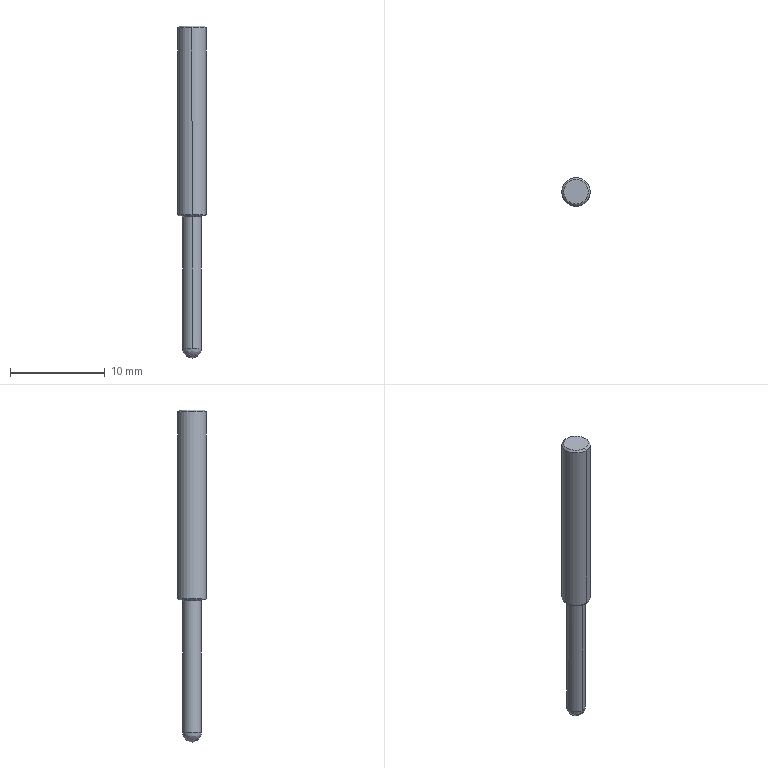Part | SolidWorks | features BaseBody 1 | 1 solid | 13 faces | box 3 x 3 x 35 mm | volume 187.251 mm3 | cone 6 | cylinder 4 | plane 2 | spline 1 | commonest cylinder face diameters 2 x2 3 x2
STEP:
#1=CARTESIAN_POINT('',(599.943,-194.552,152.402));
#2=VERTEX_POINT('',#1);
#3=CARTESIAN_POINT('',(599.943,-191.552,152.402));
#4=VERTEX_POINT('',#3);
#5=CARTESIAN_POINT('',(599.943,-193.052,152.402));
#6=DIRECTION('',(-0.000000008,0.000000019,1.));
#7=DIRECTION('',(0.,-1.,0.000000019));
#8=AXIS2_PLACEMENT_3D('',#5,#6,#7);
#9=CIRCLE('',#8,1.5);
#10=EDGE_CURVE('',#2,#4,#9,.T.);
#11=ORIENTED_EDGE('',*,*,#10,.T.);
#12=CARTESIAN_POINT('',(599.943,-191.552,172.102));
#13=VERTEX_POINT('',#12);
#14=CARTESIAN_POINT('',(599.943,-191.552,172.302));
#15=DIRECTION('',(-0.000000008,0.000000019,1.));
#16=VECTOR('',#15,1000.);
#17=LINE('',#14,#16);
#18=EDGE_CURVE('',#4,#13,#17,.T.);
#19=ORIENTED_EDGE('',*,*,#18,.T.);
#20=CARTESIAN_POINT('',(599.943,-194.552,172.102));
#21=VERTEX_POINT('',#20);
#22=CARTESIAN_POINT('',(599.943,-193.052,172.102));
#23=DIRECTION('',(0.000000008,-0.000000019,-1.));
#24=DIRECTION('',(0.,-1.,0.000000019));
#25=AXIS2_PLACEMENT_3D('',#22,#23,#24);
#26=CIRCLE('',#25,1.5);
#27=EDGE_CURVE('',#13,#21,#26,.T.);
#28=ORIENTED_EDGE('',*,*,#27,.T.);
#29=CARTESIAN_POINT('',(599.943,-194.552,172.302));
#30=DIRECTION('',(-0.000000008,0.000000019,1.));
#31=VECTOR('',#30,1000.);
#32=LINE('',#29,#31);
#33=EDGE_CURVE('',#2,#21,#32,.T.);
#34=ORIENTED_EDGE('',*,*,#33,.F.);
#35=EDGE_LOOP('',(#11,#19,#28,#34));
#36=FACE_OUTER_BOUND('',#35,.T.);
#37=CARTESIAN_POINT('',(599.943,-193.052,172.302));
#38=DIRECTION('',(-0.000000008,0.000000019,1.));
#39=DIRECTION('',(0.,-1.,0.000000019));
#40=AXIS2_PLACEMENT_3D('',#37,#38,#39);
#41=CYLINDRICAL_SURFACE('',#40,1.5);
#42=ADVANCED_FACE('',(#36),#41,.T.);
#43=CARTESIAN_POINT('',(599.943,-194.452,152.302));
#44=VERTEX_POINT('',#43);
#45=CARTESIAN_POINT('',(599.943,-191.652,152.302));
#46=VERTEX_POINT('',#45);
#47=CARTESIAN_POINT('',(599.943,-193.052,152.302));
#48=DIRECTION('',(-0.000000008,0.000000019,1.));
#49=DIRECTION('',(0.,-1.,0.000000019));
#50=AXIS2_PLACEMENT_3D('',#47,#48,#49);
#51=CIRCLE('',#50,1.4);
#52=EDGE_CURVE('',#44,#46,#51,.T.);
#53=ORIENTED_EDGE('',*,*,#52,.T.);
#54=CARTESIAN_POINT('',(599.943,-191.552,152.402));
#55=DIRECTION('',(-0.000000006,0.7071,0.7071));
#56=VECTOR('',#55,1000.);
#57=LINE('',#54,#56);
#58=EDGE_CURVE('',#46,#4,#57,.T.);
#59=ORIENTED_EDGE('',*,*,#58,.T.);
#60=ORIENTED_EDGE('',*,*,#10,.F.);
#61=CARTESIAN_POINT('',(599.943,-194.552,152.402));
#62=DIRECTION('',(-0.000000006,-0.7071,0.7071));
#63=VECTOR('',#62,1000.);
#64=LINE('',#61,#63);
#65=EDGE_CURVE('',#44,#2,#64,.T.);
#66=ORIENTED_EDGE('',*,*,#65,.F.);
#67=EDGE_LOOP('',(#53,#59,#60,#66));
#68=FACE_OUTER_BOUND('',#67,.T.);
#69=CARTESIAN_POINT('',(599.943,-193.052,152.402));
#70=DIRECTION('',(-0.000000008,0.000000019,1.));
#71=DIRECTION('',(0.,-1.,0.000000019));
#72=AXIS2_PLACEMENT_3D('',#69,#70,#71);
#73=CONICAL_SURFACE('',#72,1.5,0.7854);
#74=ADVANCED_FACE('',(#68),#73,.T.);
#75=CARTESIAN_POINT('',(599.943,-191.752,172.302));
#76=VERTEX_POINT('',#75);
#77=CARTESIAN_POINT('',(599.943,-194.352,172.302));
#78=VERTEX_POINT('',#77);
#79=CARTESIAN_POINT('',(599.943,-193.052,172.302));
#80=DIRECTION('',(0.000000008,-0.000000019,-1.));
#81=DIRECTION('',(0.,1.,-0.000000019));
#82=AXIS2_PLACEMENT_3D('',#79,#80,#81);
#83=CIRCLE('',#82,1.3);
#84=EDGE_CURVE('',#76,#78,#83,.T.);
#85=ORIENTED_EDGE('',*,*,#84,.T.);
#86=CARTESIAN_POINT('',(599.943,-194.552,172.102));
#87=DIRECTION('',(0.000000006,-0.7071,-0.7071));
#88=VECTOR('',#87,1000.);
#89=LINE('',#86,#88);
#90=EDGE_CURVE('',#78,#21,#89,.T.);
#91=ORIENTED_EDGE('',*,*,#90,.T.);
#92=ORIENTED_EDGE('',*,*,#27,.F.);
#93=CARTESIAN_POINT('',(599.943,-191.552,172.102));
#94=DIRECTION('',(0.000000006,0.7071,-0.7071));
#95=VECTOR('',#94,1000.);
#96=LINE('',#93,#95);
#97=EDGE_CURVE('',#76,#13,#96,.T.);
#98=ORIENTED_EDGE('',*,*,#97,.F.);
#99=EDGE_LOOP('',(#85,#91,#92,#98));
#100=FACE_OUTER_BOUND('',#99,.T.);
#101=CARTESIAN_POINT('',(599.943,-193.052,172.102));
#102=DIRECTION('',(0.000000008,-0.000000019,-1.));
#103=DIRECTION('',(0.,1.,-0.000000019));
#104=AXIS2_PLACEMENT_3D('',#101,#102,#103);
#105=CONICAL_SURFACE('',#104,1.5,0.7854);
#106=ADVANCED_FACE('',(#100),#105,.T.);
#107=CARTESIAN_POINT('',(599.943,-194.052,152.202));
#108=VERTEX_POINT('',#107);
#109=CARTESIAN_POINT('',(599.943,-192.052,152.202));
#110=VERTEX_POINT('',#109);
#111=CARTESIAN_POINT('',(599.943,-193.052,152.202));
#112=DIRECTION('',(-0.000000008,0.000000019,1.));
#113=DIRECTION('',(0.2216,-0.9751,0.000000021));
#114=AXIS2_PLACEMENT_3D('',#111,#112,#113);
#115=CIRCLE('',#114,1.);
#116=EDGE_CURVE('',#108,#110,#115,.T.);
#117=ORIENTED_EDGE('',*,*,#116,.T.);
#118=CARTESIAN_POINT('',(599.943,-191.952,152.302));
#119=VERTEX_POINT('',#118);
#120=CARTESIAN_POINT('',(599.943,-191.952,152.302));
#121=DIRECTION('',(-0.000000006,0.7071,0.7071));
#122=VECTOR('',#121,1000.);
#123=LINE('',#120,#122);
#124=EDGE_CURVE('',#110,#119,#123,.T.);
#125=ORIENTED_EDGE('',*,*,#124,.T.);
#126=CARTESIAN_POINT('',(599.943,-194.152,152.302));
#127=VERTEX_POINT('',#126);
#128=CARTESIAN_POINT('',(599.943,-193.052,152.302));
#129=DIRECTION('',(-0.000000008,0.000000019,1.));
#130=DIRECTION('',(0.,-1.,0.000000019));
#131=AXIS2_PLACEMENT_3D('',#128,#129,#130);
#132=CIRCLE('',#131,1.1);
#133=EDGE_CURVE('',#127,#119,#132,.T.);
#134=ORIENTED_EDGE('',*,*,#133,.F.);
#135=CARTESIAN_POINT('',(599.943,-194.152,152.302));
#136=DIRECTION('',(-0.000000006,-0.7071,0.7071));
#137=VECTOR('',#136,1000.);
#138=LINE('',#135,#137);
#139=EDGE_CURVE('',#108,#127,#138,.T.);
#140=ORIENTED_EDGE('',*,*,#139,.F.);
#141=EDGE_LOOP('',(#117,#125,#134,#140));
#142=FACE_OUTER_BOUND('',#141,.T.);
#143=CARTESIAN_POINT('',(599.943,-193.052,152.302));
#144=DIRECTION('',(-0.000000008,0.000000019,1.));
#145=DIRECTION('',(0.,-1.,0.000000019));
#146=AXIS2_PLACEMENT_3D('',#143,#144,#145);
#147=CONICAL_SURFACE('',#146,1.1,0.7854);
#148=ADVANCED_FACE('',(#142),#147,.T.);
#149=CARTESIAN_POINT('',(600.164,-194.027,138.302));
#150=VERTEX_POINT('',#149);
#151=CARTESIAN_POINT('',(599.943,-192.052,138.302));
#152=VERTEX_POINT('',#151);
#153=CARTESIAN_POINT('',(599.943,-193.052,138.302));
#154=DIRECTION('',(-0.000000008,0.000000019,1.));
#155=DIRECTION('',(0.,-1.,0.000000019));
#156=AXIS2_PLACEMENT_3D('',#153,#154,#155);
#157=CIRCLE('',#156,1.);
#158=EDGE_CURVE('',#150,#152,#157,.T.);
#159=ORIENTED_EDGE('',*,*,#158,.T.);
#160=CARTESIAN_POINT('',(599.943,-192.052,152.302));
#161=DIRECTION('',(-0.000000008,0.000000019,1.));
#162=VECTOR('',#161,1000.);
#163=LINE('',#160,#162);
#164=EDGE_CURVE('',#152,#110,#163,.T.);
#165=ORIENTED_EDGE('',*,*,#164,.T.);
#166=ORIENTED_EDGE('',*,*,#116,.F.);
#167=CARTESIAN_POINT('',(599.943,-194.052,138.302));
#168=VERTEX_POINT('',#167);
#169=CARTESIAN_POINT('',(599.943,-194.052,152.302));
#170=DIRECTION('',(-0.000000008,0.000000019,1.));
#171=VECTOR('',#170,1000.);
#172=LINE('',#169,#171);
#173=EDGE_CURVE('',#168,#108,#172,.T.);
#174=ORIENTED_EDGE('',*,*,#173,.F.);
#175=CARTESIAN_POINT('',(599.943,-193.052,138.302));
#176=DIRECTION('',(-0.000000008,0.000000019,1.));
#177=DIRECTION('',(0.,-1.,0.000000019));
#178=AXIS2_PLACEMENT_3D('',#175,#176,#177);
#179=CIRCLE('',#178,1.);
#180=EDGE_CURVE('',#168,#150,#179,.T.);
#181=ORIENTED_EDGE('',*,*,#180,.T.);
#182=EDGE_LOOP('',(#159,#165,#166,#174,#181));
#183=FACE_OUTER_BOUND('',#182,.T.);
#184=CARTESIAN_POINT('',(599.943,-193.052,152.302));
#185=DIRECTION('',(-0.000000008,0.000000019,1.));
#186=DIRECTION('',(0.,-1.,0.000000019));
#187=AXIS2_PLACEMENT_3D('',#184,#185,#186);
#188=CYLINDRICAL_SURFACE('',#187,1.);
#189=ADVANCED_FACE('',(#183),#188,.T.);
#190=ORIENTED_EDGE('',*,*,#18,.F.);
#191=CARTESIAN_POINT('',(599.943,-193.052,152.402));
#192=DIRECTION('',(-0.000000008,0.000000019,1.));
#193=DIRECTION('',(0.,-1.,0.000000019));
#194=AXIS2_PLACEMENT_3D('',#191,#192,#193);
#195=CIRCLE('',#194,1.5);
#196=EDGE_CURVE('',#4,#2,#195,.T.);
#197=ORIENTED_EDGE('',*,*,#196,.T.);
#198=ORIENTED_EDGE('',*,*,#33,.T.);
#199=CARTESIAN_POINT('',(599.943,-193.052,172.102));
#200=DIRECTION('',(0.000000008,-0.000000019,-1.));
#201=DIRECTION('',(0.,-1.,0.000000019));
#202=AXIS2_PLACEMENT_3D('',#199,#200,#201);
#203=CIRCLE('',#202,1.5);
#204=EDGE_CURVE('',#21,#13,#203,.T.);
#205=ORIENTED_EDGE('',*,*,#204,.T.);
#206=EDGE_LOOP('',(#190,#197,#198,#205));
#207=FACE_OUTER_BOUND('',#206,.T.);
#208=CARTESIAN_POINT('',(599.943,-193.052,172.302));
#209=DIRECTION('',(-0.000000008,0.000000019,1.));
#210=DIRECTION('',(0.,-1.,0.000000019));
#211=AXIS2_PLACEMENT_3D('',#208,#209,#210);
#212=CYLINDRICAL_SURFACE('',#211,1.5);
#213=ADVANCED_FACE('',(#207),#212,.T.);
#214=ORIENTED_EDGE('',*,*,#58,.F.);
#215=CARTESIAN_POINT('',(599.943,-193.052,152.302));
#216=DIRECTION('',(-0.000000008,0.000000019,1.));
#217=DIRECTION('',(0.,-1.,0.000000019));
#218=AXIS2_PLACEMENT_3D('',#215,#216,#217);
#219=CIRCLE('',#218,1.4);
#220=EDGE_CURVE('',#46,#44,#219,.T.);
#221=ORIENTED_EDGE('',*,*,#220,.T.);
#222=ORIENTED_EDGE('',*,*,#65,.T.);
#223=ORIENTED_EDGE('',*,*,#196,.F.);
#224=EDGE_LOOP('',(#214,#221,#222,#223));
#225=FACE_OUTER_BOUND('',#224,.T.);
#226=CARTESIAN_POINT('',(599.943,-193.052,152.402));
#227=DIRECTION('',(-0.000000008,0.000000019,1.));
#228=DIRECTION('',(0.,-1.,0.000000019));
#229=AXIS2_PLACEMENT_3D('',#226,#227,#228);
#230=CONICAL_SURFACE('',#229,1.5,0.7854);
#231=ADVANCED_FACE('',(#225),#230,.T.);
#232=ORIENTED_EDGE('',*,*,#90,.F.);
#233=CARTESIAN_POINT('',(599.943,-193.052,172.302));
#234=DIRECTION('',(0.000000008,-0.000000019,-1.));
#235=DIRECTION('',(0.,1.,-0.000000019));
#236=AXIS2_PLACEMENT_3D('',#233,#234,#235);
#237=CIRCLE('',#236,1.3);
#238=EDGE_CURVE('',#78,#76,#237,.T.);
#239=ORIENTED_EDGE('',*,*,#238,.T.);
#240=ORIENTED_EDGE('',*,*,#97,.T.);
#241=ORIENTED_EDGE('',*,*,#204,.F.);
#242=EDGE_LOOP('',(#232,#239,#240,#241));
#243=FACE_OUTER_BOUND('',#242,.T.);
#244=CARTESIAN_POINT('',(599.943,-193.052,172.102));
#245=DIRECTION('',(0.000000008,-0.000000019,-1.));
#246=DIRECTION('',(0.,1.,-0.000000019));
#247=AXIS2_PLACEMENT_3D('',#244,#245,#246);
#248=CONICAL_SURFACE('',#247,1.5,0.7854);
#249=ADVANCED_FACE('',(#243),#248,.T.);
#250=ORIENTED_EDGE('',*,*,#133,.T.);
#251=CARTESIAN_POINT('',(599.943,-193.052,152.302));
#252=DIRECTION('',(-0.000000008,0.000000019,1.));
#253=DIRECTION('',(0.,-1.,0.000000019));
#254=AXIS2_PLACEMENT_3D('',#251,#252,#253);
#255=CIRCLE('',#254,1.1);
#256=EDGE_CURVE('',#119,#127,#255,.T.);
#257=ORIENTED_EDGE('',*,*,#256,.T.);
#258=EDGE_LOOP('',(#250,#257));
#259=FACE_BOUND('',#258,.T.);
#260=ORIENTED_EDGE('',*,*,#52,.F.);
#261=ORIENTED_EDGE('',*,*,#220,.F.);
#262=EDGE_LOOP('',(#260,#261));
#263=FACE_OUTER_BOUND('',#262,.T.);
#264=CARTESIAN_POINT('',(599.943,-193.052,152.302));
#265=DIRECTION('',(0.000000008,-0.000000019,-1.));
#266=DIRECTION('',(0.,1.,-0.000000019));
#267=AXIS2_PLACEMENT_3D('',#264,#265,#266);
#268=PLANE('',#267);
#269=ADVANCED_FACE('',(#259,#263),#268,.T.);
#270=ORIENTED_EDGE('',*,*,#84,.F.);
#271=ORIENTED_EDGE('',*,*,#238,.F.);
#272=EDGE_LOOP('',(#270,#271));
#273=FACE_OUTER_BOUND('',#272,.T.);
#274=CARTESIAN_POINT('',(599.943,-193.052,172.302));
#275=DIRECTION('',(0.000000008,-0.000000019,-1.));
#276=DIRECTION('',(0.,1.,-0.000000019));
#277=AXIS2_PLACEMENT_3D('',#274,#275,#276);
#278=PLANE('',#277);
#279=ADVANCED_FACE('',(#273),#278,.F.);
#280=ORIENTED_EDGE('',*,*,#124,.F.);
#281=CARTESIAN_POINT('',(599.943,-193.052,152.202));
#282=DIRECTION('',(-0.000000008,0.000000019,1.));
#283=DIRECTION('',(0.2216,-0.9751,0.000000021));
#284=AXIS2_PLACEMENT_3D('',#281,#282,#283);
#285=CIRCLE('',#284,1.);
#286=EDGE_CURVE('',#110,#108,#285,.T.);
#287=ORIENTED_EDGE('',*,*,#286,.T.);
#288=ORIENTED_EDGE('',*,*,#139,.T.);
#289=ORIENTED_EDGE('',*,*,#256,.F.);
#290=EDGE_LOOP('',(#280,#287,#288,#289));
#291=FACE_OUTER_BOUND('',#290,.T.);
#292=CARTESIAN_POINT('',(599.943,-193.052,152.302));
#293=DIRECTION('',(-0.000000008,0.000000019,1.));
#294=DIRECTION('',(0.,-1.,0.000000019));
#295=AXIS2_PLACEMENT_3D('',#292,#293,#294);
#296=CONICAL_SURFACE('',#295,1.1,0.7854);
#297=ADVANCED_FACE('',(#291),#296,.T.);
#298=ORIENTED_EDGE('',*,*,#164,.F.);
#299=CARTESIAN_POINT('',(599.721,-192.076,138.302));
#300=VERTEX_POINT('',#299);
#301=CARTESIAN_POINT('',(599.943,-193.052,138.302));
#302=DIRECTION('',(-0.000000008,0.000000019,1.));
#303=DIRECTION('',(0.,-1.,0.000000019));
#304=AXIS2_PLACEMENT_3D('',#301,#302,#303);
#305=CIRCLE('',#304,1.);
#306=EDGE_CURVE('',#152,#300,#305,.T.);
#307=ORIENTED_EDGE('',*,*,#306,.T.);
#308=CARTESIAN_POINT('',(599.943,-193.052,138.302));
#309=DIRECTION('',(-0.000000008,0.000000019,1.));
#310=DIRECTION('',(0.,-1.,0.000000019));
#311=AXIS2_PLACEMENT_3D('',#308,#309,#310);
#312=CIRCLE('',#311,1.);
#313=EDGE_CURVE('',#300,#168,#312,.T.);
#314=ORIENTED_EDGE('',*,*,#313,.T.);
#315=ORIENTED_EDGE('',*,*,#173,.T.);
#316=ORIENTED_EDGE('',*,*,#286,.F.);
#317=EDGE_LOOP('',(#298,#307,#314,#315,#316));
#318=FACE_OUTER_BOUND('',#317,.T.);
#319=CARTESIAN_POINT('',(599.943,-193.052,152.302));
#320=DIRECTION('',(-0.000000008,0.000000019,1.));
#321=DIRECTION('',(0.,-1.,0.000000019));
#322=AXIS2_PLACEMENT_3D('',#319,#320,#321);
#323=CYLINDRICAL_SURFACE('',#322,1.);
#324=ADVANCED_FACE('',(#318),#323,.T.);
#325=ORIENTED_EDGE('',*,*,#313,.F.);
#326=ORIENTED_EDGE('',*,*,#306,.F.);
#327=ORIENTED_EDGE('',*,*,#158,.F.);
#328=ORIENTED_EDGE('',*,*,#180,.F.);
#329=EDGE_LOOP('',(#325,#326,#327,#328));
#330=FACE_OUTER_BOUND('',#329,.T.);
#331=CARTESIAN_POINT('',(599.721,-192.076,138.302));
#332=CARTESIAN_POINT('',(599.721,-192.076,138.302));
#333=CARTESIAN_POINT('',(599.721,-192.076,138.302));
#334=CARTESIAN_POINT('',(599.721,-192.076,138.302));
#335=CARTESIAN_POINT('',(601.671,-191.633,138.302));
#336=CARTESIAN_POINT('',(601.671,-191.633,134.302));
#337=CARTESIAN_POINT('',(597.771,-192.52,134.302));
#338=CARTESIAN_POINT('',(597.771,-192.52,138.302));
#339=CARTESIAN_POINT('',(602.115,-193.583,138.302));
#340=CARTESIAN_POINT('',(602.115,-193.583,134.302));
#341=CARTESIAN_POINT('',(598.214,-194.47,134.302));
#342=CARTESIAN_POINT('',(598.214,-194.47,138.302));
#343=CARTESIAN_POINT('',(600.164,-194.027,138.302));
#344=CARTESIAN_POINT('',(600.164,-194.027,138.302));
#345=CARTESIAN_POINT('',(600.164,-194.027,138.302));
#346=CARTESIAN_POINT('',(600.164,-194.027,138.302));
#347=(BOUNDED_SURFACE()B_SPLINE_SURFACE(3,3,((#331,#332,#333,#334),(#335,#336,#337,#338),(#339,#340,#341,#342),(#343,#344,#345,#346)),.UNSPECIFIED.,.F.,.F.,.T.)B_SPLINE_SURFACE_WITH_KNOTS((4,4),(4,4),(0.,1.),(0.,1.),.UNSPECIFIED.)GEOMETRIC_REPRESENTATION_ITEM()RATIONAL_B_SPLINE_SURFACE(((1.,0.3333,0.3333,1.),(0.3333,0.1111,0.1111,0.3333),(0.3333,0.1111,0.1111,0.3333),(1.,0.3333,0.3333,1.)))REPRESENTATION_ITEM('')SURFACE());
#348=ADVANCED_FACE('',(#330),#347,.T.);
#349=CLOSED_SHELL('',(#42,#74,#106,#148,#189,#213,#231,#249,#269,#279,#297,#324,#348));
#350=MANIFOLD_SOLID_BREP('',#349);
#351=CARTESIAN_POINT('',(0.,0.,0.));
#352=DIRECTION('',(0.,0.,1.));
#353=DIRECTION('',(1.,0.,0.));
#354=AXIS2_PLACEMENT_3D('',#351,#352,#353);
#355=(LENGTH_UNIT()NAMED_UNIT(*)SI_UNIT(.MILLI.,.METRE.));
#356=UNCERTAINTY_MEASURE_WITH_UNIT(LENGTH_MEASURE(0.00001),#355,'','');
#357=(NAMED_UNIT(*)PLANE_ANGLE_UNIT()SI_UNIT($,.RADIAN.));
#358=(NAMED_UNIT(*)SI_UNIT($,.STERADIAN.)SOLID_ANGLE_UNIT());
#359=(GEOMETRIC_REPRESENTATION_CONTEXT(3)GLOBAL_UNCERTAINTY_ASSIGNED_CONTEXT((#356))GLOBAL_UNIT_ASSIGNED_CONTEXT((#355,#357,#358))REPRESENTATION_CONTEXT('',''));
#360=ADVANCED_BREP_SHAPE_REPRESENTATION('',(#350,#354),#359);